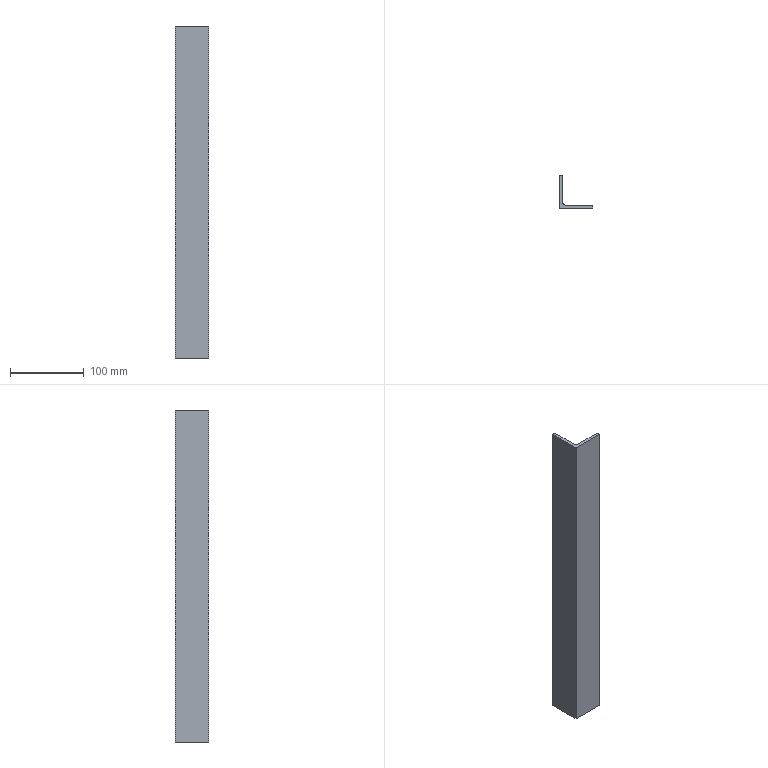Part | STEP file | 750038430 | 1 solid | 11 faces | box 45 x 45 x 450 mm | volume 156442 mm3 | plane 8 | cylinder 3 | commonest cylinder face diameters 4 x2 10 x1
STEP:
#1=CARTESIAN_POINT('',(0.,0.,225.));
#2=VERTEX_POINT('',#1);
#3=CARTESIAN_POINT('',(0.,0.,-225.));
#4=VERTEX_POINT('',#3);
#5=CARTESIAN_POINT('',(0.,0.,225.));
#6=DIRECTION('',(0.,0.,-1.));
#7=VECTOR('',#6,1000.);
#8=LINE('',#5,#7);
#9=EDGE_CURVE('',#2,#4,#8,.T.);
#10=ORIENTED_EDGE('',*,*,#9,.F.);
#11=CARTESIAN_POINT('',(0.,45.,225.));
#12=VERTEX_POINT('',#11);
#13=CARTESIAN_POINT('',(0.,45.,225.));
#14=DIRECTION('',(0.,-1.,0.));
#15=VECTOR('',#14,1000.);
#16=LINE('',#13,#15);
#17=EDGE_CURVE('',#12,#2,#16,.T.);
#18=ORIENTED_EDGE('',*,*,#17,.F.);
#19=CARTESIAN_POINT('',(0.,45.,-225.));
#20=VERTEX_POINT('',#19);
#21=CARTESIAN_POINT('',(0.,45.,225.));
#22=DIRECTION('',(0.,0.,1.));
#23=VECTOR('',#22,1000.);
#24=LINE('',#21,#23);
#25=EDGE_CURVE('',#20,#12,#24,.T.);
#26=ORIENTED_EDGE('',*,*,#25,.F.);
#27=CARTESIAN_POINT('',(0.,45.,-225.));
#28=DIRECTION('',(0.,1.,0.));
#29=VECTOR('',#28,1000.);
#30=LINE('',#27,#29);
#31=EDGE_CURVE('',#4,#20,#30,.T.);
#32=ORIENTED_EDGE('',*,*,#31,.F.);
#33=EDGE_LOOP('',(#10,#18,#26,#32));
#34=FACE_OUTER_BOUND('',#33,.T.);
#35=CARTESIAN_POINT('',(0.,45.,225.));
#36=DIRECTION('',(1.,0.,0.));
#37=DIRECTION('',(0.,0.,-1.));
#38=AXIS2_PLACEMENT_3D('',#35,#36,#37);
#39=PLANE('',#38);
#40=ADVANCED_FACE('',(#34),#39,.F.);
#41=CARTESIAN_POINT('',(2.,45.,-225.));
#42=VERTEX_POINT('',#41);
#43=CARTESIAN_POINT('',(43.,45.,-225.));
#44=DIRECTION('',(-1.,0.,0.));
#45=VECTOR('',#44,1000.);
#46=LINE('',#43,#45);
#47=EDGE_CURVE('',#42,#20,#46,.T.);
#48=ORIENTED_EDGE('',*,*,#47,.F.);
#49=CARTESIAN_POINT('',(4.,43.,-225.));
#50=VERTEX_POINT('',#49);
#51=CARTESIAN_POINT('',(2.,43.,-225.));
#52=DIRECTION('',(0.,0.,1.));
#53=DIRECTION('',(-1.,0.,0.));
#54=AXIS2_PLACEMENT_3D('',#51,#52,#53);
#55=CIRCLE('',#54,2.);
#56=EDGE_CURVE('',#50,#42,#55,.T.);
#57=ORIENTED_EDGE('',*,*,#56,.F.);
#58=CARTESIAN_POINT('',(4.,9.,-225.));
#59=VERTEX_POINT('',#58);
#60=CARTESIAN_POINT('',(4.,2.,-225.));
#61=DIRECTION('',(0.,1.,0.));
#62=VECTOR('',#61,1000.);
#63=LINE('',#60,#62);
#64=EDGE_CURVE('',#59,#50,#63,.T.);
#65=ORIENTED_EDGE('',*,*,#64,.F.);
#66=CARTESIAN_POINT('',(9.,4.,-225.));
#67=VERTEX_POINT('',#66);
#68=CARTESIAN_POINT('',(9.,9.,-225.));
#69=DIRECTION('',(0.,0.,-1.));
#70=DIRECTION('',(-1.,0.,0.));
#71=AXIS2_PLACEMENT_3D('',#68,#69,#70);
#72=CIRCLE('',#71,5.);
#73=EDGE_CURVE('',#67,#59,#72,.T.);
#74=ORIENTED_EDGE('',*,*,#73,.F.);
#75=CARTESIAN_POINT('',(43.,4.,-225.));
#76=VERTEX_POINT('',#75);
#77=CARTESIAN_POINT('',(43.,4.,-225.));
#78=DIRECTION('',(-1.,0.,0.));
#79=VECTOR('',#78,1000.);
#80=LINE('',#77,#79);
#81=EDGE_CURVE('',#76,#67,#80,.T.);
#82=ORIENTED_EDGE('',*,*,#81,.F.);
#83=CARTESIAN_POINT('',(45.,2.,-225.));
#84=VERTEX_POINT('',#83);
#85=CARTESIAN_POINT('',(43.,2.,-225.));
#86=DIRECTION('',(0.,0.,1.));
#87=DIRECTION('',(-1.,0.,0.));
#88=AXIS2_PLACEMENT_3D('',#85,#86,#87);
#89=CIRCLE('',#88,2.);
#90=EDGE_CURVE('',#84,#76,#89,.T.);
#91=ORIENTED_EDGE('',*,*,#90,.F.);
#92=CARTESIAN_POINT('',(45.,0.,-225.));
#93=VERTEX_POINT('',#92);
#94=CARTESIAN_POINT('',(45.,2.,-225.));
#95=DIRECTION('',(0.,1.,0.));
#96=VECTOR('',#95,1000.);
#97=LINE('',#94,#96);
#98=EDGE_CURVE('',#93,#84,#97,.T.);
#99=ORIENTED_EDGE('',*,*,#98,.F.);
#100=CARTESIAN_POINT('',(43.,0.,-225.));
#101=DIRECTION('',(1.,0.,0.));
#102=VECTOR('',#101,1000.);
#103=LINE('',#100,#102);
#104=EDGE_CURVE('',#4,#93,#103,.T.);
#105=ORIENTED_EDGE('',*,*,#104,.F.);
#106=ORIENTED_EDGE('',*,*,#31,.T.);
#107=EDGE_LOOP('',(#48,#57,#65,#74,#82,#91,#99,#105,#106));
#108=FACE_OUTER_BOUND('',#107,.T.);
#109=CARTESIAN_POINT('',(43.,2.,-225.));
#110=DIRECTION('',(0.,0.,1.));
#111=DIRECTION('',(1.,0.,0.));
#112=AXIS2_PLACEMENT_3D('',#109,#110,#111);
#113=PLANE('',#112);
#114=ADVANCED_FACE('',(#108),#113,.F.);
#115=CARTESIAN_POINT('',(45.,0.,225.));
#116=VERTEX_POINT('',#115);
#117=CARTESIAN_POINT('',(45.,0.,225.));
#118=DIRECTION('',(0.,0.,-1.));
#119=VECTOR('',#118,1000.);
#120=LINE('',#117,#119);
#121=EDGE_CURVE('',#116,#93,#120,.T.);
#122=ORIENTED_EDGE('',*,*,#121,.F.);
#123=CARTESIAN_POINT('',(0.,0.,225.));
#124=DIRECTION('',(1.,0.,0.));
#125=VECTOR('',#124,1000.);
#126=LINE('',#123,#125);
#127=EDGE_CURVE('',#2,#116,#126,.T.);
#128=ORIENTED_EDGE('',*,*,#127,.F.);
#129=ORIENTED_EDGE('',*,*,#9,.T.);
#130=ORIENTED_EDGE('',*,*,#104,.T.);
#131=EDGE_LOOP('',(#122,#128,#129,#130));
#132=FACE_OUTER_BOUND('',#131,.T.);
#133=CARTESIAN_POINT('',(0.,0.,225.));
#134=DIRECTION('',(0.,1.,0.));
#135=DIRECTION('',(0.,0.,1.));
#136=AXIS2_PLACEMENT_3D('',#133,#134,#135);
#137=PLANE('',#136);
#138=ADVANCED_FACE('',(#132),#137,.F.);
#139=CARTESIAN_POINT('',(4.,43.,225.));
#140=VERTEX_POINT('',#139);
#141=CARTESIAN_POINT('',(2.,45.,225.));
#142=VERTEX_POINT('',#141);
#143=CARTESIAN_POINT('',(2.,43.,225.));
#144=DIRECTION('',(0.,0.,1.));
#145=DIRECTION('',(-1.,0.,0.));
#146=AXIS2_PLACEMENT_3D('',#143,#144,#145);
#147=CIRCLE('',#146,2.);
#148=EDGE_CURVE('',#140,#142,#147,.T.);
#149=ORIENTED_EDGE('',*,*,#148,.T.);
#150=CARTESIAN_POINT('',(43.,45.,225.));
#151=DIRECTION('',(-1.,0.,0.));
#152=VECTOR('',#151,1000.);
#153=LINE('',#150,#152);
#154=EDGE_CURVE('',#142,#12,#153,.T.);
#155=ORIENTED_EDGE('',*,*,#154,.T.);
#156=ORIENTED_EDGE('',*,*,#17,.T.);
#157=ORIENTED_EDGE('',*,*,#127,.T.);
#158=CARTESIAN_POINT('',(45.,2.,225.));
#159=VERTEX_POINT('',#158);
#160=CARTESIAN_POINT('',(45.,2.,225.));
#161=DIRECTION('',(0.,1.,0.));
#162=VECTOR('',#161,1000.);
#163=LINE('',#160,#162);
#164=EDGE_CURVE('',#116,#159,#163,.T.);
#165=ORIENTED_EDGE('',*,*,#164,.T.);
#166=CARTESIAN_POINT('',(43.,4.,225.));
#167=VERTEX_POINT('',#166);
#168=CARTESIAN_POINT('',(43.,2.,225.));
#169=DIRECTION('',(0.,0.,1.));
#170=DIRECTION('',(-1.,0.,0.));
#171=AXIS2_PLACEMENT_3D('',#168,#169,#170);
#172=CIRCLE('',#171,2.);
#173=EDGE_CURVE('',#159,#167,#172,.T.);
#174=ORIENTED_EDGE('',*,*,#173,.T.);
#175=CARTESIAN_POINT('',(9.,4.,225.));
#176=VERTEX_POINT('',#175);
#177=CARTESIAN_POINT('',(43.,4.,225.));
#178=DIRECTION('',(-1.,0.,0.));
#179=VECTOR('',#178,1000.);
#180=LINE('',#177,#179);
#181=EDGE_CURVE('',#167,#176,#180,.T.);
#182=ORIENTED_EDGE('',*,*,#181,.T.);
#183=CARTESIAN_POINT('',(4.,9.,225.));
#184=VERTEX_POINT('',#183);
#185=CARTESIAN_POINT('',(9.,9.,225.));
#186=DIRECTION('',(0.,0.,-1.));
#187=DIRECTION('',(-1.,0.,0.));
#188=AXIS2_PLACEMENT_3D('',#185,#186,#187);
#189=CIRCLE('',#188,5.);
#190=EDGE_CURVE('',#176,#184,#189,.T.);
#191=ORIENTED_EDGE('',*,*,#190,.T.);
#192=CARTESIAN_POINT('',(4.,2.,225.));
#193=DIRECTION('',(0.,1.,0.));
#194=VECTOR('',#193,1000.);
#195=LINE('',#192,#194);
#196=EDGE_CURVE('',#184,#140,#195,.T.);
#197=ORIENTED_EDGE('',*,*,#196,.T.);
#198=EDGE_LOOP('',(#149,#155,#156,#157,#165,#174,#182,#191,#197));
#199=FACE_OUTER_BOUND('',#198,.T.);
#200=CARTESIAN_POINT('',(43.,2.,225.));
#201=DIRECTION('',(0.,0.,1.));
#202=DIRECTION('',(1.,0.,0.));
#203=AXIS2_PLACEMENT_3D('',#200,#201,#202);
#204=PLANE('',#203);
#205=ADVANCED_FACE('',(#199),#204,.T.);
#206=ORIENTED_EDGE('',*,*,#25,.T.);
#207=ORIENTED_EDGE('',*,*,#154,.F.);
#208=CARTESIAN_POINT('',(2.,45.,225.));
#209=DIRECTION('',(0.,0.,1.));
#210=VECTOR('',#209,1000.);
#211=LINE('',#208,#210);
#212=EDGE_CURVE('',#42,#142,#211,.T.);
#213=ORIENTED_EDGE('',*,*,#212,.F.);
#214=ORIENTED_EDGE('',*,*,#47,.T.);
#215=EDGE_LOOP('',(#206,#207,#213,#214));
#216=FACE_OUTER_BOUND('',#215,.T.);
#217=CARTESIAN_POINT('',(2.,45.,225.));
#218=DIRECTION('',(0.,-1.,0.));
#219=DIRECTION('',(0.,0.,-1.));
#220=AXIS2_PLACEMENT_3D('',#217,#218,#219);
#221=PLANE('',#220);
#222=ADVANCED_FACE('',(#216),#221,.F.);
#223=ORIENTED_EDGE('',*,*,#148,.F.);
#224=CARTESIAN_POINT('',(4.,43.,225.));
#225=DIRECTION('',(0.,0.,-1.));
#226=VECTOR('',#225,1000.);
#227=LINE('',#224,#226);
#228=EDGE_CURVE('',#140,#50,#227,.T.);
#229=ORIENTED_EDGE('',*,*,#228,.T.);
#230=ORIENTED_EDGE('',*,*,#56,.T.);
#231=ORIENTED_EDGE('',*,*,#212,.T.);
#232=EDGE_LOOP('',(#223,#229,#230,#231));
#233=FACE_OUTER_BOUND('',#232,.T.);
#234=CARTESIAN_POINT('',(2.,43.,225.));
#235=DIRECTION('',(0.,0.,-1.));
#236=DIRECTION('',(-1.,0.,0.));
#237=AXIS2_PLACEMENT_3D('',#234,#235,#236);
#238=CYLINDRICAL_SURFACE('',#237,2.);
#239=ADVANCED_FACE('',(#233),#238,.T.);
#240=ORIENTED_EDGE('',*,*,#228,.F.);
#241=ORIENTED_EDGE('',*,*,#196,.F.);
#242=CARTESIAN_POINT('',(4.,9.,225.));
#243=DIRECTION('',(0.,0.,1.));
#244=VECTOR('',#243,1000.);
#245=LINE('',#242,#244);
#246=EDGE_CURVE('',#59,#184,#245,.T.);
#247=ORIENTED_EDGE('',*,*,#246,.F.);
#248=ORIENTED_EDGE('',*,*,#64,.T.);
#249=EDGE_LOOP('',(#240,#241,#247,#248));
#250=FACE_OUTER_BOUND('',#249,.T.);
#251=CARTESIAN_POINT('',(4.,9.,225.));
#252=DIRECTION('',(-1.,0.,0.));
#253=DIRECTION('',(0.,-1.,0.));
#254=AXIS2_PLACEMENT_3D('',#251,#252,#253);
#255=PLANE('',#254);
#256=ADVANCED_FACE('',(#250),#255,.F.);
#257=ORIENTED_EDGE('',*,*,#246,.T.);
#258=ORIENTED_EDGE('',*,*,#190,.F.);
#259=CARTESIAN_POINT('',(9.,4.,225.));
#260=DIRECTION('',(0.,0.,1.));
#261=VECTOR('',#260,1000.);
#262=LINE('',#259,#261);
#263=EDGE_CURVE('',#67,#176,#262,.T.);
#264=ORIENTED_EDGE('',*,*,#263,.F.);
#265=ORIENTED_EDGE('',*,*,#73,.T.);
#266=EDGE_LOOP('',(#257,#258,#264,#265));
#267=FACE_OUTER_BOUND('',#266,.T.);
#268=CARTESIAN_POINT('',(9.,9.,225.));
#269=DIRECTION('',(0.,0.,-1.));
#270=DIRECTION('',(-1.,0.,0.));
#271=AXIS2_PLACEMENT_3D('',#268,#269,#270);
#272=CYLINDRICAL_SURFACE('',#271,5.);
#273=ADVANCED_FACE('',(#267),#272,.F.);
#274=ORIENTED_EDGE('',*,*,#263,.T.);
#275=ORIENTED_EDGE('',*,*,#181,.F.);
#276=CARTESIAN_POINT('',(43.,4.,225.));
#277=DIRECTION('',(0.,0.,1.));
#278=VECTOR('',#277,1000.);
#279=LINE('',#276,#278);
#280=EDGE_CURVE('',#76,#167,#279,.T.);
#281=ORIENTED_EDGE('',*,*,#280,.F.);
#282=ORIENTED_EDGE('',*,*,#81,.T.);
#283=EDGE_LOOP('',(#274,#275,#281,#282));
#284=FACE_OUTER_BOUND('',#283,.T.);
#285=CARTESIAN_POINT('',(43.,4.,225.));
#286=DIRECTION('',(0.,-1.,0.));
#287=DIRECTION('',(1.,0.,0.));
#288=AXIS2_PLACEMENT_3D('',#285,#286,#287);
#289=PLANE('',#288);
#290=ADVANCED_FACE('',(#284),#289,.F.);
#291=ORIENTED_EDGE('',*,*,#173,.F.);
#292=CARTESIAN_POINT('',(45.,2.,225.));
#293=DIRECTION('',(0.,0.,-1.));
#294=VECTOR('',#293,1000.);
#295=LINE('',#292,#294);
#296=EDGE_CURVE('',#159,#84,#295,.T.);
#297=ORIENTED_EDGE('',*,*,#296,.T.);
#298=ORIENTED_EDGE('',*,*,#90,.T.);
#299=ORIENTED_EDGE('',*,*,#280,.T.);
#300=EDGE_LOOP('',(#291,#297,#298,#299));
#301=FACE_OUTER_BOUND('',#300,.T.);
#302=CARTESIAN_POINT('',(43.,2.,225.));
#303=DIRECTION('',(0.,0.,-1.));
#304=DIRECTION('',(-1.,0.,0.));
#305=AXIS2_PLACEMENT_3D('',#302,#303,#304);
#306=CYLINDRICAL_SURFACE('',#305,2.);
#307=ADVANCED_FACE('',(#301),#306,.T.);
#308=ORIENTED_EDGE('',*,*,#296,.F.);
#309=ORIENTED_EDGE('',*,*,#164,.F.);
#310=ORIENTED_EDGE('',*,*,#121,.T.);
#311=ORIENTED_EDGE('',*,*,#98,.T.);
#312=EDGE_LOOP('',(#308,#309,#310,#311));
#313=FACE_OUTER_BOUND('',#312,.T.);
#314=CARTESIAN_POINT('',(45.,0.,225.));
#315=DIRECTION('',(-1.,0.,0.));
#316=DIRECTION('',(0.,0.,1.));
#317=AXIS2_PLACEMENT_3D('',#314,#315,#316);
#318=PLANE('',#317);
#319=ADVANCED_FACE('',(#313),#318,.F.);
#320=CLOSED_SHELL('',(#40,#114,#138,#205,#222,#239,#256,#273,#290,#307,#319));
#321=MANIFOLD_SOLID_BREP('',#320);
#322=CARTESIAN_POINT('',(0.,0.,0.));
#323=DIRECTION('',(0.,0.,1.));
#324=DIRECTION('',(1.,0.,0.));
#325=AXIS2_PLACEMENT_3D('',#322,#323,#324);
#326=(LENGTH_UNIT()NAMED_UNIT(*)SI_UNIT(.MILLI.,.METRE.));
#327=UNCERTAINTY_MEASURE_WITH_UNIT(LENGTH_MEASURE(0.00001),#326,'','');
#328=(NAMED_UNIT(*)PLANE_ANGLE_UNIT()SI_UNIT($,.RADIAN.));
#329=(NAMED_UNIT(*)SI_UNIT($,.STERADIAN.)SOLID_ANGLE_UNIT());
#330=(GEOMETRIC_REPRESENTATION_CONTEXT(3)GLOBAL_UNCERTAINTY_ASSIGNED_CONTEXT((#327))GLOBAL_UNIT_ASSIGNED_CONTEXT((#326,#328,#329))REPRESENTATION_CONTEXT('',''));
#331=ADVANCED_BREP_SHAPE_REPRESENTATION('',(#321,#325),#330);